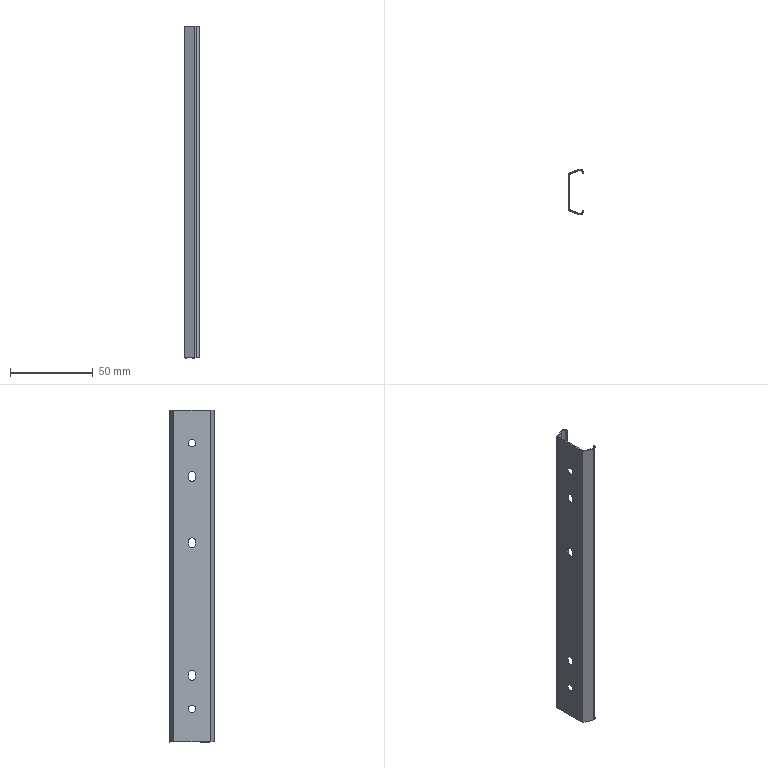Part | SolidWorks | features BaseBody 1 | 1 solid | 37 faces | box 9 x 27 x 200 mm | volume 4310 mm3 | plane 20 | cylinder 17 | commonest cylinder face diameters 4.2 x9 3.7 x4 4.5 x4
STEP:
#1=CARTESIAN_POINT('',(-2.5,11.15,17.75));
#2=VERTEX_POINT('',#1);
#3=CARTESIAN_POINT('',(-2.5,11.15,22.25));
#4=VERTEX_POINT('',#3);
#5=CARTESIAN_POINT('',(-2.5,11.15,20.));
#6=DIRECTION('',(-1.,0.,0.));
#7=DIRECTION('',(0.,0.,1.));
#8=AXIS2_PLACEMENT_3D('',#5,#6,#7);
#9=CIRCLE('',#8,2.25);
#10=EDGE_CURVE('',#2,#4,#9,.T.);
#11=ORIENTED_EDGE('',*,*,#10,.F.);
#12=CARTESIAN_POINT('',(-3.,11.15,17.75));
#13=VERTEX_POINT('',#12);
#14=CARTESIAN_POINT('',(-3.,11.15,17.75));
#15=DIRECTION('',(-1.,0.,0.));
#16=VECTOR('',#15,1000.);
#17=LINE('',#14,#16);
#18=EDGE_CURVE('',#2,#13,#17,.T.);
#19=ORIENTED_EDGE('',*,*,#18,.T.);
#20=CARTESIAN_POINT('',(-3.,11.15,22.25));
#21=VERTEX_POINT('',#20);
#22=CARTESIAN_POINT('',(-3.,11.15,20.));
#23=DIRECTION('',(1.,0.,0.));
#24=DIRECTION('',(0.,0.,1.));
#25=AXIS2_PLACEMENT_3D('',#22,#23,#24);
#26=CIRCLE('',#25,2.25);
#27=EDGE_CURVE('',#21,#13,#26,.T.);
#28=ORIENTED_EDGE('',*,*,#27,.F.);
#29=CARTESIAN_POINT('',(-3.,11.15,22.25));
#30=DIRECTION('',(-1.,0.,0.));
#31=VECTOR('',#30,1000.);
#32=LINE('',#29,#31);
#33=EDGE_CURVE('',#4,#21,#32,.T.);
#34=ORIENTED_EDGE('',*,*,#33,.F.);
#35=EDGE_LOOP('',(#11,#19,#28,#34));
#36=FACE_OUTER_BOUND('',#35,.T.);
#37=CARTESIAN_POINT('',(-3.,11.15,20.));
#38=DIRECTION('',(-1.,0.,0.));
#39=DIRECTION('',(0.,0.,1.));
#40=AXIS2_PLACEMENT_3D('',#37,#38,#39);
#41=CYLINDRICAL_SURFACE('',#40,2.25);
#42=ADVANCED_FACE('',(#36),#41,.F.);
#43=CARTESIAN_POINT('',(-2.5,11.15,177.75));
#44=VERTEX_POINT('',#43);
#45=CARTESIAN_POINT('',(-2.5,11.15,182.25));
#46=VERTEX_POINT('',#45);
#47=CARTESIAN_POINT('',(-2.5,11.15,180.));
#48=DIRECTION('',(-1.,0.,0.));
#49=DIRECTION('',(0.,0.,1.));
#50=AXIS2_PLACEMENT_3D('',#47,#48,#49);
#51=CIRCLE('',#50,2.25);
#52=EDGE_CURVE('',#44,#46,#51,.T.);
#53=ORIENTED_EDGE('',*,*,#52,.F.);
#54=CARTESIAN_POINT('',(-3.,11.15,177.75));
#55=VERTEX_POINT('',#54);
#56=CARTESIAN_POINT('',(-3.,11.15,177.75));
#57=DIRECTION('',(-1.,0.,0.));
#58=VECTOR('',#57,1000.);
#59=LINE('',#56,#58);
#60=EDGE_CURVE('',#44,#55,#59,.T.);
#61=ORIENTED_EDGE('',*,*,#60,.T.);
#62=CARTESIAN_POINT('',(-3.,11.15,182.25));
#63=VERTEX_POINT('',#62);
#64=CARTESIAN_POINT('',(-3.,11.15,180.));
#65=DIRECTION('',(1.,0.,0.));
#66=DIRECTION('',(0.,0.,1.));
#67=AXIS2_PLACEMENT_3D('',#64,#65,#66);
#68=CIRCLE('',#67,2.25);
#69=EDGE_CURVE('',#63,#55,#68,.T.);
#70=ORIENTED_EDGE('',*,*,#69,.F.);
#71=CARTESIAN_POINT('',(-3.,11.15,182.25));
#72=DIRECTION('',(-1.,0.,0.));
#73=VECTOR('',#72,1000.);
#74=LINE('',#71,#73);
#75=EDGE_CURVE('',#46,#63,#74,.T.);
#76=ORIENTED_EDGE('',*,*,#75,.F.);
#77=EDGE_LOOP('',(#53,#61,#70,#76));
#78=FACE_OUTER_BOUND('',#77,.T.);
#79=CARTESIAN_POINT('',(-3.,11.15,180.));
#80=DIRECTION('',(-1.,0.,0.));
#81=DIRECTION('',(0.,0.,1.));
#82=AXIS2_PLACEMENT_3D('',#79,#80,#81);
#83=CYLINDRICAL_SURFACE('',#82,2.25);
#84=ADVANCED_FACE('',(#78),#83,.F.);
#85=CARTESIAN_POINT('',(-2.5,11.15,43.));
#86=VERTEX_POINT('',#85);
#87=CARTESIAN_POINT('',(-2.5,13.25,40.9));
#88=VERTEX_POINT('',#87);
#89=CARTESIAN_POINT('',(-2.5,11.15,40.9));
#90=DIRECTION('',(-1.,0.,0.));
#91=DIRECTION('',(0.,0.,1.));
#92=AXIS2_PLACEMENT_3D('',#89,#90,#91);
#93=CIRCLE('',#92,2.1);
#94=EDGE_CURVE('',#86,#88,#93,.T.);
#95=ORIENTED_EDGE('',*,*,#94,.F.);
#96=CARTESIAN_POINT('',(-3.,11.15,43.));
#97=VERTEX_POINT('',#96);
#98=CARTESIAN_POINT('',(-3.,11.15,43.));
#99=DIRECTION('',(-1.,0.,0.));
#100=VECTOR('',#99,1000.);
#101=LINE('',#98,#100);
#102=EDGE_CURVE('',#86,#97,#101,.T.);
#103=ORIENTED_EDGE('',*,*,#102,.T.);
#104=CARTESIAN_POINT('',(-3.,13.25,40.9));
#105=VERTEX_POINT('',#104);
#106=CARTESIAN_POINT('',(-3.,11.15,40.9));
#107=DIRECTION('',(1.,0.,0.));
#108=DIRECTION('',(0.,0.,1.));
#109=AXIS2_PLACEMENT_3D('',#106,#107,#108);
#110=CIRCLE('',#109,2.1);
#111=EDGE_CURVE('',#105,#97,#110,.T.);
#112=ORIENTED_EDGE('',*,*,#111,.F.);
#113=CARTESIAN_POINT('',(-3.,13.25,40.9));
#114=DIRECTION('',(-1.,0.,0.));
#115=VECTOR('',#114,1000.);
#116=LINE('',#113,#115);
#117=EDGE_CURVE('',#88,#105,#116,.T.);
#118=ORIENTED_EDGE('',*,*,#117,.F.);
#119=EDGE_LOOP('',(#95,#103,#112,#118));
#120=FACE_OUTER_BOUND('',#119,.T.);
#121=CARTESIAN_POINT('',(-3.,11.15,40.9));
#122=DIRECTION('',(-1.,0.,0.));
#123=DIRECTION('',(0.,0.,1.));
#124=AXIS2_PLACEMENT_3D('',#121,#122,#123);
#125=CYLINDRICAL_SURFACE('',#124,2.1);
#126=ADVANCED_FACE('',(#120),#125,.F.);
#127=CARTESIAN_POINT('',(-2.5,11.15,163.));
#128=VERTEX_POINT('',#127);
#129=CARTESIAN_POINT('',(-2.5,13.25,160.9));
#130=VERTEX_POINT('',#129);
#131=CARTESIAN_POINT('',(-2.5,11.15,160.9));
#132=DIRECTION('',(-1.,0.,0.));
#133=DIRECTION('',(0.,0.,1.));
#134=AXIS2_PLACEMENT_3D('',#131,#132,#133);
#135=CIRCLE('',#134,2.1);
#136=EDGE_CURVE('',#128,#130,#135,.T.);
#137=ORIENTED_EDGE('',*,*,#136,.F.);
#138=CARTESIAN_POINT('',(-3.,11.15,163.));
#139=VERTEX_POINT('',#138);
#140=CARTESIAN_POINT('',(-3.,11.15,163.));
#141=DIRECTION('',(-1.,0.,0.));
#142=VECTOR('',#141,1000.);
#143=LINE('',#140,#142);
#144=EDGE_CURVE('',#128,#139,#143,.T.);
#145=ORIENTED_EDGE('',*,*,#144,.T.);
#146=CARTESIAN_POINT('',(-3.,13.25,160.9));
#147=VERTEX_POINT('',#146);
#148=CARTESIAN_POINT('',(-3.,11.15,160.9));
#149=DIRECTION('',(1.,0.,0.));
#150=DIRECTION('',(0.,0.,1.));
#151=AXIS2_PLACEMENT_3D('',#148,#149,#150);
#152=CIRCLE('',#151,2.1);
#153=EDGE_CURVE('',#147,#139,#152,.T.);
#154=ORIENTED_EDGE('',*,*,#153,.F.);
#155=CARTESIAN_POINT('',(-3.,13.25,160.9));
#156=DIRECTION('',(-1.,0.,0.));
#157=VECTOR('',#156,1000.);
#158=LINE('',#155,#157);
#159=EDGE_CURVE('',#130,#147,#158,.T.);
#160=ORIENTED_EDGE('',*,*,#159,.F.);
#161=EDGE_LOOP('',(#137,#145,#154,#160));
#162=FACE_OUTER_BOUND('',#161,.T.);
#163=CARTESIAN_POINT('',(-3.,11.15,160.9));
#164=DIRECTION('',(-1.,0.,0.));
#165=DIRECTION('',(0.,0.,1.));
#166=AXIS2_PLACEMENT_3D('',#163,#164,#165);
#167=CYLINDRICAL_SURFACE('',#166,2.1);
#168=ADVANCED_FACE('',(#162),#167,.F.);
#169=CARTESIAN_POINT('',(-2.5,11.15,123.));
#170=VERTEX_POINT('',#169);
#171=CARTESIAN_POINT('',(-2.5,13.25,120.9));
#172=VERTEX_POINT('',#171);
#173=CARTESIAN_POINT('',(-2.5,11.15,120.9));
#174=DIRECTION('',(-1.,0.,0.));
#175=DIRECTION('',(0.,0.,1.));
#176=AXIS2_PLACEMENT_3D('',#173,#174,#175);
#177=CIRCLE('',#176,2.1);
#178=EDGE_CURVE('',#170,#172,#177,.T.);
#179=ORIENTED_EDGE('',*,*,#178,.F.);
#180=CARTESIAN_POINT('',(-3.,11.15,123.));
#181=VERTEX_POINT('',#180);
#182=CARTESIAN_POINT('',(-3.,11.15,123.));
#183=DIRECTION('',(-1.,0.,0.));
#184=VECTOR('',#183,1000.);
#185=LINE('',#182,#184);
#186=EDGE_CURVE('',#170,#181,#185,.T.);
#187=ORIENTED_EDGE('',*,*,#186,.T.);
#188=CARTESIAN_POINT('',(-3.,13.25,120.9));
#189=VERTEX_POINT('',#188);
#190=CARTESIAN_POINT('',(-3.,11.15,120.9));
#191=DIRECTION('',(1.,0.,0.));
#192=DIRECTION('',(0.,0.,1.));
#193=AXIS2_PLACEMENT_3D('',#190,#191,#192);
#194=CIRCLE('',#193,2.1);
#195=EDGE_CURVE('',#189,#181,#194,.T.);
#196=ORIENTED_EDGE('',*,*,#195,.F.);
#197=CARTESIAN_POINT('',(-3.,13.25,120.9));
#198=DIRECTION('',(-1.,0.,0.));
#199=VECTOR('',#198,1000.);
#200=LINE('',#197,#199);
#201=EDGE_CURVE('',#172,#189,#200,.T.);
#202=ORIENTED_EDGE('',*,*,#201,.F.);
#203=EDGE_LOOP('',(#179,#187,#196,#202));
#204=FACE_OUTER_BOUND('',#203,.T.);
#205=CARTESIAN_POINT('',(-3.,11.15,120.9));
#206=DIRECTION('',(-1.,0.,0.));
#207=DIRECTION('',(0.,0.,1.));
#208=AXIS2_PLACEMENT_3D('',#205,#206,#207);
#209=CYLINDRICAL_SURFACE('',#208,2.1);
#210=ADVANCED_FACE('',(#204),#209,.F.);
#211=CARTESIAN_POINT('',(-3.,0.05325,200.));
#212=VERTEX_POINT('',#211);
#213=CARTESIAN_POINT('',(-3.,22.247,200.));
#214=VERTEX_POINT('',#213);
#215=CARTESIAN_POINT('',(-3.,22.247,200.));
#216=DIRECTION('',(0.,1.,0.));
#217=VECTOR('',#216,1000.);
#218=LINE('',#215,#217);
#219=EDGE_CURVE('',#212,#214,#218,.T.);
#220=ORIENTED_EDGE('',*,*,#219,.T.);
#221=CARTESIAN_POINT('',(-3.,22.247,0.));
#222=VERTEX_POINT('',#221);
#223=CARTESIAN_POINT('',(-3.,22.247,200.));
#224=DIRECTION('',(0.,0.,-1.));
#225=VECTOR('',#224,1000.);
#226=LINE('',#223,#225);
#227=EDGE_CURVE('',#214,#222,#226,.T.);
#228=ORIENTED_EDGE('',*,*,#227,.T.);
#229=CARTESIAN_POINT('',(-3.,0.05325,0.));
#230=VERTEX_POINT('',#229);
#231=CARTESIAN_POINT('',(-3.,22.247,0.));
#232=DIRECTION('',(0.,-1.,0.));
#233=VECTOR('',#232,1000.);
#234=LINE('',#231,#233);
#235=EDGE_CURVE('',#222,#230,#234,.T.);
#236=ORIENTED_EDGE('',*,*,#235,.T.);
#237=CARTESIAN_POINT('',(-3.,0.05325,200.));
#238=DIRECTION('',(0.,0.,1.));
#239=VECTOR('',#238,1000.);
#240=LINE('',#237,#239);
#241=EDGE_CURVE('',#230,#212,#240,.T.);
#242=ORIENTED_EDGE('',*,*,#241,.T.);
#243=EDGE_LOOP('',(#220,#228,#236,#242));
#244=FACE_OUTER_BOUND('',#243,.T.);
#245=ORIENTED_EDGE('',*,*,#27,.T.);
#246=CARTESIAN_POINT('',(-3.,11.15,20.));
#247=DIRECTION('',(1.,0.,0.));
#248=DIRECTION('',(0.,0.,1.));
#249=AXIS2_PLACEMENT_3D('',#246,#247,#248);
#250=CIRCLE('',#249,2.25);
#251=EDGE_CURVE('',#13,#21,#250,.T.);
#252=ORIENTED_EDGE('',*,*,#251,.T.);
#253=EDGE_LOOP('',(#245,#252));
#254=FACE_BOUND('',#253,.T.);
#255=ORIENTED_EDGE('',*,*,#69,.T.);
#256=CARTESIAN_POINT('',(-3.,11.15,180.));
#257=DIRECTION('',(1.,0.,0.));
#258=DIRECTION('',(0.,0.,1.));
#259=AXIS2_PLACEMENT_3D('',#256,#257,#258);
#260=CIRCLE('',#259,2.25);
#261=EDGE_CURVE('',#55,#63,#260,.T.);
#262=ORIENTED_EDGE('',*,*,#261,.T.);
#263=EDGE_LOOP('',(#255,#262));
#264=FACE_BOUND('',#263,.T.);
#265=ORIENTED_EDGE('',*,*,#111,.T.);
#266=CARTESIAN_POINT('',(-3.,9.05,40.9));
#267=VERTEX_POINT('',#266);
#268=CARTESIAN_POINT('',(-3.,11.15,40.9));
#269=DIRECTION('',(1.,0.,0.));
#270=DIRECTION('',(0.,0.,1.));
#271=AXIS2_PLACEMENT_3D('',#268,#269,#270);
#272=CIRCLE('',#271,2.1);
#273=EDGE_CURVE('',#97,#267,#272,.T.);
#274=ORIENTED_EDGE('',*,*,#273,.T.);
#275=CARTESIAN_POINT('',(-3.,9.05,39.1));
#276=VERTEX_POINT('',#275);
#277=CARTESIAN_POINT('',(-3.,9.05,200.));
#278=DIRECTION('',(0.,0.,-1.));
#279=VECTOR('',#278,1000.);
#280=LINE('',#277,#279);
#281=EDGE_CURVE('',#267,#276,#280,.T.);
#282=ORIENTED_EDGE('',*,*,#281,.T.);
#283=CARTESIAN_POINT('',(-3.,13.25,39.1));
#284=VERTEX_POINT('',#283);
#285=CARTESIAN_POINT('',(-3.,11.15,39.1));
#286=DIRECTION('',(1.,0.,0.));
#287=DIRECTION('',(0.,0.,1.));
#288=AXIS2_PLACEMENT_3D('',#285,#286,#287);
#289=CIRCLE('',#288,2.1);
#290=EDGE_CURVE('',#276,#284,#289,.T.);
#291=ORIENTED_EDGE('',*,*,#290,.T.);
#292=CARTESIAN_POINT('',(-3.,13.25,200.));
#293=DIRECTION('',(0.,0.,1.));
#294=VECTOR('',#293,1000.);
#295=LINE('',#292,#294);
#296=EDGE_CURVE('',#284,#105,#295,.T.);
#297=ORIENTED_EDGE('',*,*,#296,.T.);
#298=EDGE_LOOP('',(#265,#274,#282,#291,#297));
#299=FACE_BOUND('',#298,.T.);
#300=ORIENTED_EDGE('',*,*,#153,.T.);
#301=CARTESIAN_POINT('',(-3.,9.05,160.9));
#302=VERTEX_POINT('',#301);
#303=CARTESIAN_POINT('',(-3.,11.15,160.9));
#304=DIRECTION('',(1.,0.,0.));
#305=DIRECTION('',(0.,0.,1.));
#306=AXIS2_PLACEMENT_3D('',#303,#304,#305);
#307=CIRCLE('',#306,2.1);
#308=EDGE_CURVE('',#139,#302,#307,.T.);
#309=ORIENTED_EDGE('',*,*,#308,.T.);
#310=CARTESIAN_POINT('',(-3.,9.05,159.1));
#311=VERTEX_POINT('',#310);
#312=CARTESIAN_POINT('',(-3.,9.05,200.));
#313=DIRECTION('',(0.,0.,-1.));
#314=VECTOR('',#313,1000.);
#315=LINE('',#312,#314);
#316=EDGE_CURVE('',#302,#311,#315,.T.);
#317=ORIENTED_EDGE('',*,*,#316,.T.);
#318=CARTESIAN_POINT('',(-3.,13.25,159.1));
#319=VERTEX_POINT('',#318);
#320=CARTESIAN_POINT('',(-3.,11.15,159.1));
#321=DIRECTION('',(1.,0.,0.));
#322=DIRECTION('',(0.,0.,1.));
#323=AXIS2_PLACEMENT_3D('',#320,#321,#322);
#324=CIRCLE('',#323,2.1);
#325=EDGE_CURVE('',#311,#319,#324,.T.);
#326=ORIENTED_EDGE('',*,*,#325,.T.);
#327=CARTESIAN_POINT('',(-3.,13.25,200.));
#328=DIRECTION('',(0.,0.,1.));
#329=VECTOR('',#328,1000.);
#330=LINE('',#327,#329);
#331=EDGE_CURVE('',#319,#147,#330,.T.);
#332=ORIENTED_EDGE('',*,*,#331,.T.);
#333=EDGE_LOOP('',(#300,#309,#317,#326,#332));
#334=FACE_BOUND('',#333,.T.);
#335=ORIENTED_EDGE('',*,*,#195,.T.);
#336=CARTESIAN_POINT('',(-3.,9.05,120.9));
#337=VERTEX_POINT('',#336);
#338=CARTESIAN_POINT('',(-3.,11.15,120.9));
#339=DIRECTION('',(1.,0.,0.));
#340=DIRECTION('',(0.,0.,1.));
#341=AXIS2_PLACEMENT_3D('',#338,#339,#340);
#342=CIRCLE('',#341,2.1);
#343=EDGE_CURVE('',#181,#337,#342,.T.);
#344=ORIENTED_EDGE('',*,*,#343,.T.);
#345=CARTESIAN_POINT('',(-3.,9.05,119.1));
#346=VERTEX_POINT('',#345);
#347=CARTESIAN_POINT('',(-3.,9.05,200.));
#348=DIRECTION('',(0.,0.,-1.));
#349=VECTOR('',#348,1000.);
#350=LINE('',#347,#349);
#351=EDGE_CURVE('',#337,#346,#350,.T.);
#352=ORIENTED_EDGE('',*,*,#351,.T.);
#353=CARTESIAN_POINT('',(-3.,13.25,119.1));
#354=VERTEX_POINT('',#353);
#355=CARTESIAN_POINT('',(-3.,11.15,119.1));
#356=DIRECTION('',(1.,0.,0.));
#357=DIRECTION('',(0.,0.,1.));
#358=AXIS2_PLACEMENT_3D('',#355,#356,#357);
#359=CIRCLE('',#358,2.1);
#360=EDGE_CURVE('',#346,#354,#359,.T.);
#361=ORIENTED_EDGE('',*,*,#360,.T.);
#362=CARTESIAN_POINT('',(-3.,13.25,200.));
#363=DIRECTION('',(0.,0.,1.));
#364=VECTOR('',#363,1000.);
#365=LINE('',#362,#364);
#366=EDGE_CURVE('',#354,#189,#365,.T.);
#367=ORIENTED_EDGE('',*,*,#366,.T.);
#368=EDGE_LOOP('',(#335,#344,#352,#361,#367));
#369=FACE_BOUND('',#368,.T.);
#370=CARTESIAN_POINT('',(-3.,22.247,200.));
#371=DIRECTION('',(-1.,0.,0.));
#372=DIRECTION('',(0.,0.,1.));
#373=AXIS2_PLACEMENT_3D('',#370,#371,#372);
#374=PLANE('',#373);
#375=ADVANCED_FACE('',(#244,#254,#264,#299,#334,#369),#374,.T.);
#376=CARTESIAN_POINT('',(3.211,24.65,200.));
#377=VERTEX_POINT('',#376);
#378=CARTESIAN_POINT('',(3.211,24.65,200.));
#379=DIRECTION('',(0.9326,0.3609,0.));
#380=VECTOR('',#379,1000.);
#381=LINE('',#378,#380);
#382=EDGE_CURVE('',#214,#377,#381,.T.);
#383=ORIENTED_EDGE('',*,*,#382,.T.);
#384=CARTESIAN_POINT('',(3.211,24.65,0.));
#385=VERTEX_POINT('',#384);
#386=CARTESIAN_POINT('',(3.211,24.65,200.));
#387=DIRECTION('',(0.,0.,-1.));
#388=VECTOR('',#387,1000.);
#389=LINE('',#386,#388);
#390=EDGE_CURVE('',#377,#385,#389,.T.);
#391=ORIENTED_EDGE('',*,*,#390,.T.);
#392=CARTESIAN_POINT('',(3.211,24.65,0.));
#393=DIRECTION('',(-0.9326,-0.3609,0.));
#394=VECTOR('',#393,1000.);
#395=LINE('',#392,#394);
#396=EDGE_CURVE('',#385,#222,#395,.T.);
#397=ORIENTED_EDGE('',*,*,#396,.T.);
#398=ORIENTED_EDGE('',*,*,#227,.F.);
#399=EDGE_LOOP('',(#383,#391,#397,#398));
#400=FACE_OUTER_BOUND('',#399,.T.);
#401=CARTESIAN_POINT('',(3.211,24.65,200.));
#402=DIRECTION('',(-0.3609,0.9326,0.));
#403=DIRECTION('',(-0.9326,-0.3609,0.));
#404=AXIS2_PLACEMENT_3D('',#401,#402,#403);
#405=PLANE('',#404);
#406=ADVANCED_FACE('',(#400),#405,.T.);
#407=CARTESIAN_POINT('',(3.211,-2.35,200.));
#408=VERTEX_POINT('',#407);
#409=CARTESIAN_POINT('',(3.211,-2.35,200.));
#410=DIRECTION('',(-0.9326,0.3609,0.));
#411=VECTOR('',#410,1000.);
#412=LINE('',#409,#411);
#413=EDGE_CURVE('',#408,#212,#412,.T.);
#414=ORIENTED_EDGE('',*,*,#413,.F.);
#415=CARTESIAN_POINT('',(4.15,-2.35,200.));
#416=VERTEX_POINT('',#415);
#417=CARTESIAN_POINT('',(3.211,-2.35,200.));
#418=DIRECTION('',(-1.,0.,0.));
#419=VECTOR('',#418,1000.);
#420=LINE('',#417,#419);
#421=EDGE_CURVE('',#416,#408,#420,.T.);
#422=ORIENTED_EDGE('',*,*,#421,.F.);
#423=CARTESIAN_POINT('',(6.,-0.5,200.));
#424=VERTEX_POINT('',#423);
#425=CARTESIAN_POINT('',(4.15,-0.5,200.));
#426=DIRECTION('',(0.,0.,-1.));
#427=DIRECTION('',(1.,0.,0.));
#428=AXIS2_PLACEMENT_3D('',#425,#426,#427);
#429=CIRCLE('',#428,1.85);
#430=EDGE_CURVE('',#424,#416,#429,.T.);
#431=ORIENTED_EDGE('',*,*,#430,.F.);
#432=CARTESIAN_POINT('',(6.,-0.2056,200.));
#433=VERTEX_POINT('',#432);
#434=CARTESIAN_POINT('',(6.,-0.5,200.));
#435=DIRECTION('',(0.,-1.,0.));
#436=VECTOR('',#435,1000.);
#437=LINE('',#434,#436);
#438=EDGE_CURVE('',#433,#424,#437,.T.);
#439=ORIENTED_EDGE('',*,*,#438,.F.);
#440=CARTESIAN_POINT('',(5.493,-0.1612,200.));
#441=VERTEX_POINT('',#440);
#442=CARTESIAN_POINT('',(6.,-0.2056,200.));
#443=DIRECTION('',(0.9962,-0.08716,0.));
#444=VECTOR('',#443,1000.);
#445=LINE('',#442,#444);
#446=EDGE_CURVE('',#441,#433,#445,.T.);
#447=ORIENTED_EDGE('',*,*,#446,.F.);
#448=CARTESIAN_POINT('',(2.982,-1.725,200.));
#449=VERTEX_POINT('',#448);
#450=CARTESIAN_POINT('',(3.65,0.,200.));
#451=DIRECTION('',(0.,0.,1.));
#452=DIRECTION('',(1.,0.,0.));
#453=AXIS2_PLACEMENT_3D('',#450,#451,#452);
#454=CIRCLE('',#453,1.85);
#455=EDGE_CURVE('',#449,#441,#454,.T.);
#456=ORIENTED_EDGE('',*,*,#455,.F.);
#457=CARTESIAN_POINT('',(-2.5,0.3959,200.));
#458=VERTEX_POINT('',#457);
#459=CARTESIAN_POINT('',(-2.5,0.3959,200.));
#460=DIRECTION('',(0.9326,-0.3609,0.));
#461=VECTOR('',#460,1000.);
#462=LINE('',#459,#461);
#463=EDGE_CURVE('',#458,#449,#462,.T.);
#464=ORIENTED_EDGE('',*,*,#463,.F.);
#465=CARTESIAN_POINT('',(-2.5,21.904,200.));
#466=VERTEX_POINT('',#465);
#467=CARTESIAN_POINT('',(-2.5,24.65,200.));
#468=DIRECTION('',(0.,-1.,0.));
#469=VECTOR('',#468,1000.);
#470=LINE('',#467,#469);
#471=EDGE_CURVE('',#466,#458,#470,.T.);
#472=ORIENTED_EDGE('',*,*,#471,.F.);
#473=CARTESIAN_POINT('',(2.982,24.025,200.));
#474=VERTEX_POINT('',#473);
#475=CARTESIAN_POINT('',(2.982,24.025,200.));
#476=DIRECTION('',(-0.9326,-0.3609,0.));
#477=VECTOR('',#476,1000.);
#478=LINE('',#475,#477);
#479=EDGE_CURVE('',#474,#466,#478,.T.);
#480=ORIENTED_EDGE('',*,*,#479,.F.);
#481=CARTESIAN_POINT('',(5.493,22.461,200.));
#482=VERTEX_POINT('',#481);
#483=CARTESIAN_POINT('',(3.65,22.3,200.));
#484=DIRECTION('',(0.,0.,1.));
#485=DIRECTION('',(1.,0.,0.));
#486=AXIS2_PLACEMENT_3D('',#483,#484,#485);
#487=CIRCLE('',#486,1.85);
#488=EDGE_CURVE('',#482,#474,#487,.T.);
#489=ORIENTED_EDGE('',*,*,#488,.F.);
#490=CARTESIAN_POINT('',(6.,22.506,200.));
#491=VERTEX_POINT('',#490);
#492=CARTESIAN_POINT('',(5.493,22.461,200.));
#493=DIRECTION('',(-0.9962,-0.08716,0.));
#494=VECTOR('',#493,1000.);
#495=LINE('',#492,#494);
#496=EDGE_CURVE('',#491,#482,#495,.T.);
#497=ORIENTED_EDGE('',*,*,#496,.F.);
#498=CARTESIAN_POINT('',(6.,22.8,200.));
#499=VERTEX_POINT('',#498);
#500=CARTESIAN_POINT('',(6.,22.506,200.));
#501=DIRECTION('',(0.,-1.,0.));
#502=VECTOR('',#501,1000.);
#503=LINE('',#500,#502);
#504=EDGE_CURVE('',#499,#491,#503,.T.);
#505=ORIENTED_EDGE('',*,*,#504,.F.);
#506=CARTESIAN_POINT('',(4.15,24.65,200.));
#507=VERTEX_POINT('',#506);
#508=CARTESIAN_POINT('',(4.15,22.8,200.));
#509=DIRECTION('',(0.,0.,-1.));
#510=DIRECTION('',(1.,0.,0.));
#511=AXIS2_PLACEMENT_3D('',#508,#509,#510);
#512=CIRCLE('',#511,1.85);
#513=EDGE_CURVE('',#507,#499,#512,.T.);
#514=ORIENTED_EDGE('',*,*,#513,.F.);
#515=CARTESIAN_POINT('',(-3.,24.65,200.));
#516=DIRECTION('',(1.,0.,0.));
#517=VECTOR('',#516,1000.);
#518=LINE('',#515,#517);
#519=EDGE_CURVE('',#377,#507,#518,.T.);
#520=ORIENTED_EDGE('',*,*,#519,.F.);
#521=ORIENTED_EDGE('',*,*,#382,.F.);
#522=ORIENTED_EDGE('',*,*,#219,.F.);
#523=EDGE_LOOP('',(#414,#422,#431,#439,#447,#456,#464,#472,#480,#489,#497,#505,#514,#520,#521,#522));
#524=FACE_OUTER_BOUND('',#523,.T.);
#525=CARTESIAN_POINT('',(-3.,24.65,200.));
#526=DIRECTION('',(0.,0.,-1.));
#527=DIRECTION('',(-1.,0.,0.));
#528=AXIS2_PLACEMENT_3D('',#525,#526,#527);
#529=PLANE('',#528);
#530=ADVANCED_FACE('',(#524),#529,.F.);
#531=ORIENTED_EDGE('',*,*,#413,.T.);
#532=ORIENTED_EDGE('',*,*,#241,.F.);
#533=CARTESIAN_POINT('',(3.211,-2.35,0.));
#534=VERTEX_POINT('',#533);
#535=CARTESIAN_POINT('',(-3.,0.05325,0.));
#536=DIRECTION('',(0.9326,-0.3609,0.));
#537=VECTOR('',#536,1000.);
#538=LINE('',#535,#537);
#539=EDGE_CURVE('',#230,#534,#538,.T.);
#540=ORIENTED_EDGE('',*,*,#539,.T.);
#541=CARTESIAN_POINT('',(3.211,-2.35,200.));
#542=DIRECTION('',(0.,0.,1.));
#543=VECTOR('',#542,1000.);
#544=LINE('',#541,#543);
#545=EDGE_CURVE('',#534,#408,#544,.T.);
#546=ORIENTED_EDGE('',*,*,#545,.T.);
#547=EDGE_LOOP('',(#531,#532,#540,#546));
#548=FACE_OUTER_BOUND('',#547,.T.);
#549=CARTESIAN_POINT('',(-3.,0.05325,200.));
#550=DIRECTION('',(-0.3609,-0.9326,0.));
#551=DIRECTION('',(0.9326,-0.3609,0.));
#552=AXIS2_PLACEMENT_3D('',#549,#550,#551);
#553=PLANE('',#552);
#554=ADVANCED_FACE('',(#548),#553,.T.);
#555=CARTESIAN_POINT('',(6.,-0.5,0.));
#556=VERTEX_POINT('',#555);
#557=CARTESIAN_POINT('',(4.15,-2.35,0.));
#558=VERTEX_POINT('',#557);
#559=CARTESIAN_POINT('',(4.15,-0.5,0.));
#560=DIRECTION('',(0.,0.,-1.));
#561=DIRECTION('',(1.,0.,0.));
#562=AXIS2_PLACEMENT_3D('',#559,#560,#561);
#563=CIRCLE('',#562,1.85);
#564=EDGE_CURVE('',#556,#558,#563,.T.);
#565=ORIENTED_EDGE('',*,*,#564,.T.);
#566=CARTESIAN_POINT('',(-3.,-2.35,0.));
#567=DIRECTION('',(-1.,0.,0.));
#568=VECTOR('',#567,1000.);
#569=LINE('',#566,#568);
#570=EDGE_CURVE('',#558,#534,#569,.T.);
#571=ORIENTED_EDGE('',*,*,#570,.T.);
#572=ORIENTED_EDGE('',*,*,#539,.F.);
#573=ORIENTED_EDGE('',*,*,#235,.F.);
#574=ORIENTED_EDGE('',*,*,#396,.F.);
#575=CARTESIAN_POINT('',(4.15,24.65,0.));
#576=VERTEX_POINT('',#575);
#577=CARTESIAN_POINT('',(-3.,24.65,0.));
#578=DIRECTION('',(1.,0.,0.));
#579=VECTOR('',#578,1000.);
#580=LINE('',#577,#579);
#581=EDGE_CURVE('',#385,#576,#580,.T.);
#582=ORIENTED_EDGE('',*,*,#581,.T.);
#583=CARTESIAN_POINT('',(6.,22.8,0.));
#584=VERTEX_POINT('',#583);
#585=CARTESIAN_POINT('',(4.15,22.8,0.));
#586=DIRECTION('',(0.,0.,-1.));
#587=DIRECTION('',(1.,0.,0.));
#588=AXIS2_PLACEMENT_3D('',#585,#586,#587);
#589=CIRCLE('',#588,1.85);
#590=EDGE_CURVE('',#576,#584,#589,.T.);
#591=ORIENTED_EDGE('',*,*,#590,.T.);
#592=CARTESIAN_POINT('',(6.,22.506,0.));
#593=VERTEX_POINT('',#592);
#594=CARTESIAN_POINT('',(6.,22.506,0.));
#595=DIRECTION('',(0.,1.,0.));
#596=VECTOR('',#595,1000.);
#597=LINE('',#594,#596);
#598=EDGE_CURVE('',#593,#584,#597,.T.);
#599=ORIENTED_EDGE('',*,*,#598,.F.);
#600=CARTESIAN_POINT('',(5.493,22.461,0.));
#601=VERTEX_POINT('',#600);
#602=CARTESIAN_POINT('',(5.493,22.461,0.));
#603=DIRECTION('',(0.9962,0.08716,0.));
#604=VECTOR('',#603,1000.);
#605=LINE('',#602,#604);
#606=EDGE_CURVE('',#601,#593,#605,.T.);
#607=ORIENTED_EDGE('',*,*,#606,.F.);
#608=CARTESIAN_POINT('',(2.982,24.025,0.));
#609=VERTEX_POINT('',#608);
#610=CARTESIAN_POINT('',(3.65,22.3,0.));
#611=DIRECTION('',(0.,0.,1.));
#612=DIRECTION('',(1.,0.,0.));
#613=AXIS2_PLACEMENT_3D('',#610,#611,#612);
#614=CIRCLE('',#613,1.85);
#615=EDGE_CURVE('',#601,#609,#614,.T.);
#616=ORIENTED_EDGE('',*,*,#615,.T.);
#617=CARTESIAN_POINT('',(-2.5,21.904,0.));
#618=VERTEX_POINT('',#617);
#619=CARTESIAN_POINT('',(2.982,24.025,0.));
#620=DIRECTION('',(-0.9326,-0.3609,0.));
#621=VECTOR('',#620,1000.);
#622=LINE('',#619,#621);
#623=EDGE_CURVE('',#609,#618,#622,.T.);
#624=ORIENTED_EDGE('',*,*,#623,.T.);
#625=CARTESIAN_POINT('',(-2.5,0.3959,0.));
#626=VERTEX_POINT('',#625);
#627=CARTESIAN_POINT('',(-2.5,24.65,0.));
#628=DIRECTION('',(0.,-1.,0.));
#629=VECTOR('',#628,1000.);
#630=LINE('',#627,#629);
#631=EDGE_CURVE('',#618,#626,#630,.T.);
#632=ORIENTED_EDGE('',*,*,#631,.T.);
#633=CARTESIAN_POINT('',(2.982,-1.725,0.));
#634=VERTEX_POINT('',#633);
#635=CARTESIAN_POINT('',(-2.5,0.3959,0.));
#636=DIRECTION('',(0.9326,-0.3609,0.));
#637=VECTOR('',#636,1000.);
#638=LINE('',#635,#637);
#639=EDGE_CURVE('',#626,#634,#638,.T.);
#640=ORIENTED_EDGE('',*,*,#639,.T.);
#641=CARTESIAN_POINT('',(5.493,-0.1612,0.));
#642=VERTEX_POINT('',#641);
#643=CARTESIAN_POINT('',(3.65,0.,0.));
#644=DIRECTION('',(0.,0.,1.));
#645=DIRECTION('',(1.,0.,0.));
#646=AXIS2_PLACEMENT_3D('',#643,#644,#645);
#647=CIRCLE('',#646,1.85);
#648=EDGE_CURVE('',#634,#642,#647,.T.);
#649=ORIENTED_EDGE('',*,*,#648,.T.);
#650=CARTESIAN_POINT('',(6.,-0.2056,0.));
#651=VERTEX_POINT('',#650);
#652=CARTESIAN_POINT('',(6.,-0.2056,0.));
#653=DIRECTION('',(-0.9962,0.08716,0.));
#654=VECTOR('',#653,1000.);
#655=LINE('',#652,#654);
#656=EDGE_CURVE('',#651,#642,#655,.T.);
#657=ORIENTED_EDGE('',*,*,#656,.F.);
#658=CARTESIAN_POINT('',(6.,-0.5,0.));
#659=DIRECTION('',(0.,1.,0.));
#660=VECTOR('',#659,1000.);
#661=LINE('',#658,#660);
#662=EDGE_CURVE('',#556,#651,#661,.T.);
#663=ORIENTED_EDGE('',*,*,#662,.F.);
#664=EDGE_LOOP('',(#565,#571,#572,#573,#574,#582,#591,#599,#607,#616,#624,#632,#640,#649,#657,#663));
#665=FACE_OUTER_BOUND('',#664,.T.);
#666=CARTESIAN_POINT('',(-3.,24.65,0.));
#667=DIRECTION('',(0.,0.,-1.));
#668=DIRECTION('',(-1.,0.,0.));
#669=AXIS2_PLACEMENT_3D('',#666,#667,#668);
#670=PLANE('',#669);
#671=ADVANCED_FACE('',(#665),#670,.T.);
#672=ORIENTED_EDGE('',*,*,#18,.F.);
#673=CARTESIAN_POINT('',(-2.5,11.15,20.));
#674=DIRECTION('',(-1.,0.,0.));
#675=DIRECTION('',(0.,0.,1.));
#676=AXIS2_PLACEMENT_3D('',#673,#674,#675);
#677=CIRCLE('',#676,2.25);
#678=EDGE_CURVE('',#4,#2,#677,.T.);
#679=ORIENTED_EDGE('',*,*,#678,.F.);
#680=ORIENTED_EDGE('',*,*,#33,.T.);
#681=ORIENTED_EDGE('',*,*,#251,.F.);
#682=EDGE_LOOP('',(#672,#679,#680,#681));
#683=FACE_OUTER_BOUND('',#682,.T.);
#684=CARTESIAN_POINT('',(-3.,11.15,20.));
#685=DIRECTION('',(-1.,0.,0.));
#686=DIRECTION('',(0.,0.,1.));
#687=AXIS2_PLACEMENT_3D('',#684,#685,#686);
#688=CYLINDRICAL_SURFACE('',#687,2.25);
#689=ADVANCED_FACE('',(#683),#688,.F.);
#690=ORIENTED_EDGE('',*,*,#60,.F.);
#691=CARTESIAN_POINT('',(-2.5,11.15,180.));
#692=DIRECTION('',(-1.,0.,0.));
#693=DIRECTION('',(0.,0.,1.));
#694=AXIS2_PLACEMENT_3D('',#691,#692,#693);
#695=CIRCLE('',#694,2.25);
#696=EDGE_CURVE('',#46,#44,#695,.T.);
#697=ORIENTED_EDGE('',*,*,#696,.F.);
#698=ORIENTED_EDGE('',*,*,#75,.T.);
#699=ORIENTED_EDGE('',*,*,#261,.F.);
#700=EDGE_LOOP('',(#690,#697,#698,#699));
#701=FACE_OUTER_BOUND('',#700,.T.);
#702=CARTESIAN_POINT('',(-3.,11.15,180.));
#703=DIRECTION('',(-1.,0.,0.));
#704=DIRECTION('',(0.,0.,1.));
#705=AXIS2_PLACEMENT_3D('',#702,#703,#704);
#706=CYLINDRICAL_SURFACE('',#705,2.25);
#707=ADVANCED_FACE('',(#701),#706,.F.);
#708=CARTESIAN_POINT('',(-2.5,9.05,39.1));
#709=VERTEX_POINT('',#708);
#710=CARTESIAN_POINT('',(-3.,9.05,39.1));
#711=DIRECTION('',(1.,0.,0.));
#712=VECTOR('',#711,1000.);
#713=LINE('',#710,#712);
#714=EDGE_CURVE('',#276,#709,#713,.T.);
#715=ORIENTED_EDGE('',*,*,#714,.F.);
#716=ORIENTED_EDGE('',*,*,#281,.F.);
#717=CARTESIAN_POINT('',(-2.5,9.05,40.9));
#718=VERTEX_POINT('',#717);
#719=CARTESIAN_POINT('',(-3.,9.05,40.9));
#720=DIRECTION('',(-1.,0.,0.));
#721=VECTOR('',#720,1000.);
#722=LINE('',#719,#721);
#723=EDGE_CURVE('',#718,#267,#722,.T.);
#724=ORIENTED_EDGE('',*,*,#723,.F.);
#725=CARTESIAN_POINT('',(-2.5,9.05,39.1));
#726=DIRECTION('',(0.,0.,1.));
#727=VECTOR('',#726,1000.);
#728=LINE('',#725,#727);
#729=EDGE_CURVE('',#709,#718,#728,.T.);
#730=ORIENTED_EDGE('',*,*,#729,.F.);
#731=EDGE_LOOP('',(#715,#716,#724,#730));
#732=FACE_OUTER_BOUND('',#731,.T.);
#733=CARTESIAN_POINT('',(-3.,9.05,39.1));
#734=DIRECTION('',(0.,-1.,0.));
#735=DIRECTION('',(0.,0.,-1.));
#736=AXIS2_PLACEMENT_3D('',#733,#734,#735);
#737=PLANE('',#736);
#738=ADVANCED_FACE('',(#732),#737,.F.);
#739=ORIENTED_EDGE('',*,*,#102,.F.);
#740=CARTESIAN_POINT('',(-2.5,11.15,40.9));
#741=DIRECTION('',(-1.,0.,0.));
#742=DIRECTION('',(0.,0.,1.));
#743=AXIS2_PLACEMENT_3D('',#740,#741,#742);
#744=CIRCLE('',#743,2.1);
#745=EDGE_CURVE('',#718,#86,#744,.T.);
#746=ORIENTED_EDGE('',*,*,#745,.F.);
#747=ORIENTED_EDGE('',*,*,#723,.T.);
#748=ORIENTED_EDGE('',*,*,#273,.F.);
#749=EDGE_LOOP('',(#739,#746,#747,#748));
#750=FACE_OUTER_BOUND('',#749,.T.);
#751=CARTESIAN_POINT('',(-3.,11.15,40.9));
#752=DIRECTION('',(-1.,0.,0.));
#753=DIRECTION('',(0.,0.,1.));
#754=AXIS2_PLACEMENT_3D('',#751,#752,#753);
#755=CYLINDRICAL_SURFACE('',#754,2.1);
#756=ADVANCED_FACE('',(#750),#755,.F.);
#757=ORIENTED_EDGE('',*,*,#117,.T.);
#758=ORIENTED_EDGE('',*,*,#296,.F.);
#759=CARTESIAN_POINT('',(-2.5,13.25,39.1));
#760=VERTEX_POINT('',#759);
#761=CARTESIAN_POINT('',(-3.,13.25,39.1));
#762=DIRECTION('',(-1.,0.,0.));
#763=VECTOR('',#762,1000.);
#764=LINE('',#761,#763);
#765=EDGE_CURVE('',#760,#284,#764,.T.);
#766=ORIENTED_EDGE('',*,*,#765,.F.);
#767=CARTESIAN_POINT('',(-2.5,13.25,40.9));
#768=DIRECTION('',(0.,0.,-1.));
#769=VECTOR('',#768,1000.);
#770=LINE('',#767,#769);
#771=EDGE_CURVE('',#88,#760,#770,.T.);
#772=ORIENTED_EDGE('',*,*,#771,.F.);
#773=EDGE_LOOP('',(#757,#758,#766,#772));
#774=FACE_OUTER_BOUND('',#773,.T.);
#775=CARTESIAN_POINT('',(-3.,13.25,40.9));
#776=DIRECTION('',(0.,1.,0.));
#777=DIRECTION('',(0.,0.,1.));
#778=AXIS2_PLACEMENT_3D('',#775,#776,#777);
#779=PLANE('',#778);
#780=ADVANCED_FACE('',(#774),#779,.F.);
#781=ORIENTED_EDGE('',*,*,#765,.T.);
#782=ORIENTED_EDGE('',*,*,#290,.F.);
#783=ORIENTED_EDGE('',*,*,#714,.T.);
#784=CARTESIAN_POINT('',(-2.5,11.15,39.1));
#785=DIRECTION('',(-1.,0.,0.));
#786=DIRECTION('',(0.,0.,1.));
#787=AXIS2_PLACEMENT_3D('',#784,#785,#786);
#788=CIRCLE('',#787,2.1);
#789=EDGE_CURVE('',#760,#709,#788,.T.);
#790=ORIENTED_EDGE('',*,*,#789,.F.);
#791=EDGE_LOOP('',(#781,#782,#783,#790));
#792=FACE_OUTER_BOUND('',#791,.T.);
#793=CARTESIAN_POINT('',(-3.,11.15,39.1));
#794=DIRECTION('',(-1.,0.,0.));
#795=DIRECTION('',(0.,0.,1.));
#796=AXIS2_PLACEMENT_3D('',#793,#794,#795);
#797=CYLINDRICAL_SURFACE('',#796,2.1);
#798=ADVANCED_FACE('',(#792),#797,.F.);
#799=CARTESIAN_POINT('',(-2.5,9.05,159.1));
#800=VERTEX_POINT('',#799);
#801=CARTESIAN_POINT('',(-3.,9.05,159.1));
#802=DIRECTION('',(1.,0.,0.));
#803=VECTOR('',#802,1000.);
#804=LINE('',#801,#803);
#805=EDGE_CURVE('',#311,#800,#804,.T.);
#806=ORIENTED_EDGE('',*,*,#805,.F.);
#807=ORIENTED_EDGE('',*,*,#316,.F.);
#808=CARTESIAN_POINT('',(-2.5,9.05,160.9));
#809=VERTEX_POINT('',#808);
#810=CARTESIAN_POINT('',(-3.,9.05,160.9));
#811=DIRECTION('',(-1.,0.,0.));
#812=VECTOR('',#811,1000.);
#813=LINE('',#810,#812);
#814=EDGE_CURVE('',#809,#302,#813,.T.);
#815=ORIENTED_EDGE('',*,*,#814,.F.);
#816=CARTESIAN_POINT('',(-2.5,9.05,159.1));
#817=DIRECTION('',(0.,0.,1.));
#818=VECTOR('',#817,1000.);
#819=LINE('',#816,#818);
#820=EDGE_CURVE('',#800,#809,#819,.T.);
#821=ORIENTED_EDGE('',*,*,#820,.F.);
#822=EDGE_LOOP('',(#806,#807,#815,#821));
#823=FACE_OUTER_BOUND('',#822,.T.);
#824=CARTESIAN_POINT('',(-3.,9.05,159.1));
#825=DIRECTION('',(0.,-1.,0.));
#826=DIRECTION('',(0.,0.,-1.));
#827=AXIS2_PLACEMENT_3D('',#824,#825,#826);
#828=PLANE('',#827);
#829=ADVANCED_FACE('',(#823),#828,.F.);
#830=ORIENTED_EDGE('',*,*,#144,.F.);
#831=CARTESIAN_POINT('',(-2.5,11.15,160.9));
#832=DIRECTION('',(-1.,0.,0.));
#833=DIRECTION('',(0.,0.,1.));
#834=AXIS2_PLACEMENT_3D('',#831,#832,#833);
#835=CIRCLE('',#834,2.1);
#836=EDGE_CURVE('',#809,#128,#835,.T.);
#837=ORIENTED_EDGE('',*,*,#836,.F.);
#838=ORIENTED_EDGE('',*,*,#814,.T.);
#839=ORIENTED_EDGE('',*,*,#308,.F.);
#840=EDGE_LOOP('',(#830,#837,#838,#839));
#841=FACE_OUTER_BOUND('',#840,.T.);
#842=CARTESIAN_POINT('',(-3.,11.15,160.9));
#843=DIRECTION('',(-1.,0.,0.));
#844=DIRECTION('',(0.,0.,1.));
#845=AXIS2_PLACEMENT_3D('',#842,#843,#844);
#846=CYLINDRICAL_SURFACE('',#845,2.1);
#847=ADVANCED_FACE('',(#841),#846,.F.);
#848=ORIENTED_EDGE('',*,*,#159,.T.);
#849=ORIENTED_EDGE('',*,*,#331,.F.);
#850=CARTESIAN_POINT('',(-2.5,13.25,159.1));
#851=VERTEX_POINT('',#850);
#852=CARTESIAN_POINT('',(-3.,13.25,159.1));
#853=DIRECTION('',(-1.,0.,0.));
#854=VECTOR('',#853,1000.);
#855=LINE('',#852,#854);
#856=EDGE_CURVE('',#851,#319,#855,.T.);
#857=ORIENTED_EDGE('',*,*,#856,.F.);
#858=CARTESIAN_POINT('',(-2.5,13.25,160.9));
#859=DIRECTION('',(0.,0.,-1.));
#860=VECTOR('',#859,1000.);
#861=LINE('',#858,#860);
#862=EDGE_CURVE('',#130,#851,#861,.T.);
#863=ORIENTED_EDGE('',*,*,#862,.F.);
#864=EDGE_LOOP('',(#848,#849,#857,#863));
#865=FACE_OUTER_BOUND('',#864,.T.);
#866=CARTESIAN_POINT('',(-3.,13.25,160.9));
#867=DIRECTION('',(0.,1.,0.));
#868=DIRECTION('',(0.,0.,1.));
#869=AXIS2_PLACEMENT_3D('',#866,#867,#868);
#870=PLANE('',#869);
#871=ADVANCED_FACE('',(#865),#870,.F.);
#872=ORIENTED_EDGE('',*,*,#856,.T.);
#873=ORIENTED_EDGE('',*,*,#325,.F.);
#874=ORIENTED_EDGE('',*,*,#805,.T.);
#875=CARTESIAN_POINT('',(-2.5,11.15,159.1));
#876=DIRECTION('',(-1.,0.,0.));
#877=DIRECTION('',(0.,0.,1.));
#878=AXIS2_PLACEMENT_3D('',#875,#876,#877);
#879=CIRCLE('',#878,2.1);
#880=EDGE_CURVE('',#851,#800,#879,.T.);
#881=ORIENTED_EDGE('',*,*,#880,.F.);
#882=EDGE_LOOP('',(#872,#873,#874,#881));
#883=FACE_OUTER_BOUND('',#882,.T.);
#884=CARTESIAN_POINT('',(-3.,11.15,159.1));
#885=DIRECTION('',(-1.,0.,0.));
#886=DIRECTION('',(0.,0.,1.));
#887=AXIS2_PLACEMENT_3D('',#884,#885,#886);
#888=CYLINDRICAL_SURFACE('',#887,2.1);
#889=ADVANCED_FACE('',(#883),#888,.F.);
#890=CARTESIAN_POINT('',(-2.5,9.05,119.1));
#891=VERTEX_POINT('',#890);
#892=CARTESIAN_POINT('',(-3.,9.05,119.1));
#893=DIRECTION('',(1.,0.,0.));
#894=VECTOR('',#893,1000.);
#895=LINE('',#892,#894);
#896=EDGE_CURVE('',#346,#891,#895,.T.);
#897=ORIENTED_EDGE('',*,*,#896,.F.);
#898=ORIENTED_EDGE('',*,*,#351,.F.);
#899=CARTESIAN_POINT('',(-2.5,9.05,120.9));
#900=VERTEX_POINT('',#899);
#901=CARTESIAN_POINT('',(-3.,9.05,120.9));
#902=DIRECTION('',(-1.,0.,0.));
#903=VECTOR('',#902,1000.);
#904=LINE('',#901,#903);
#905=EDGE_CURVE('',#900,#337,#904,.T.);
#906=ORIENTED_EDGE('',*,*,#905,.F.);
#907=CARTESIAN_POINT('',(-2.5,9.05,119.1));
#908=DIRECTION('',(0.,0.,1.));
#909=VECTOR('',#908,1000.);
#910=LINE('',#907,#909);
#911=EDGE_CURVE('',#891,#900,#910,.T.);
#912=ORIENTED_EDGE('',*,*,#911,.F.);
#913=EDGE_LOOP('',(#897,#898,#906,#912));
#914=FACE_OUTER_BOUND('',#913,.T.);
#915=CARTESIAN_POINT('',(-3.,9.05,119.1));
#916=DIRECTION('',(0.,-1.,0.));
#917=DIRECTION('',(0.,0.,-1.));
#918=AXIS2_PLACEMENT_3D('',#915,#916,#917);
#919=PLANE('',#918);
#920=ADVANCED_FACE('',(#914),#919,.F.);
#921=ORIENTED_EDGE('',*,*,#186,.F.);
#922=CARTESIAN_POINT('',(-2.5,11.15,120.9));
#923=DIRECTION('',(-1.,0.,0.));
#924=DIRECTION('',(0.,0.,1.));
#925=AXIS2_PLACEMENT_3D('',#922,#923,#924);
#926=CIRCLE('',#925,2.1);
#927=EDGE_CURVE('',#900,#170,#926,.T.);
#928=ORIENTED_EDGE('',*,*,#927,.F.);
#929=ORIENTED_EDGE('',*,*,#905,.T.);
#930=ORIENTED_EDGE('',*,*,#343,.F.);
#931=EDGE_LOOP('',(#921,#928,#929,#930));
#932=FACE_OUTER_BOUND('',#931,.T.);
#933=CARTESIAN_POINT('',(-3.,11.15,120.9));
#934=DIRECTION('',(-1.,0.,0.));
#935=DIRECTION('',(0.,0.,1.));
#936=AXIS2_PLACEMENT_3D('',#933,#934,#935);
#937=CYLINDRICAL_SURFACE('',#936,2.1);
#938=ADVANCED_FACE('',(#932),#937,.F.);
#939=ORIENTED_EDGE('',*,*,#201,.T.);
#940=ORIENTED_EDGE('',*,*,#366,.F.);
#941=CARTESIAN_POINT('',(-2.5,13.25,119.1));
#942=VERTEX_POINT('',#941);
#943=CARTESIAN_POINT('',(-3.,13.25,119.1));
#944=DIRECTION('',(-1.,0.,0.));
#945=VECTOR('',#944,1000.);
#946=LINE('',#943,#945);
#947=EDGE_CURVE('',#942,#354,#946,.T.);
#948=ORIENTED_EDGE('',*,*,#947,.F.);
#949=CARTESIAN_POINT('',(-2.5,13.25,120.9));
#950=DIRECTION('',(0.,0.,-1.));
#951=VECTOR('',#950,1000.);
#952=LINE('',#949,#951);
#953=EDGE_CURVE('',#172,#942,#952,.T.);
#954=ORIENTED_EDGE('',*,*,#953,.F.);
#955=EDGE_LOOP('',(#939,#940,#948,#954));
#956=FACE_OUTER_BOUND('',#955,.T.);
#957=CARTESIAN_POINT('',(-3.,13.25,120.9));
#958=DIRECTION('',(0.,1.,0.));
#959=DIRECTION('',(0.,0.,1.));
#960=AXIS2_PLACEMENT_3D('',#957,#958,#959);
#961=PLANE('',#960);
#962=ADVANCED_FACE('',(#956),#961,.F.);
#963=ORIENTED_EDGE('',*,*,#947,.T.);
#964=ORIENTED_EDGE('',*,*,#360,.F.);
#965=ORIENTED_EDGE('',*,*,#896,.T.);
#966=CARTESIAN_POINT('',(-2.5,11.15,119.1));
#967=DIRECTION('',(-1.,0.,0.));
#968=DIRECTION('',(0.,0.,1.));
#969=AXIS2_PLACEMENT_3D('',#966,#967,#968);
#970=CIRCLE('',#969,2.1);
#971=EDGE_CURVE('',#942,#891,#970,.T.);
#972=ORIENTED_EDGE('',*,*,#971,.F.);
#973=EDGE_LOOP('',(#963,#964,#965,#972));
#974=FACE_OUTER_BOUND('',#973,.T.);
#975=CARTESIAN_POINT('',(-3.,11.15,119.1));
#976=DIRECTION('',(-1.,0.,0.));
#977=DIRECTION('',(0.,0.,1.));
#978=AXIS2_PLACEMENT_3D('',#975,#976,#977);
#979=CYLINDRICAL_SURFACE('',#978,2.1);
#980=ADVANCED_FACE('',(#974),#979,.F.);
#981=ORIENTED_EDGE('',*,*,#519,.T.);
#982=CARTESIAN_POINT('',(4.15,24.65,200.));
#983=DIRECTION('',(0.,0.,-1.));
#984=VECTOR('',#983,1000.);
#985=LINE('',#982,#984);
#986=EDGE_CURVE('',#507,#576,#985,.T.);
#987=ORIENTED_EDGE('',*,*,#986,.T.);
#988=ORIENTED_EDGE('',*,*,#581,.F.);
#989=ORIENTED_EDGE('',*,*,#390,.F.);
#990=EDGE_LOOP('',(#981,#987,#988,#989));
#991=FACE_OUTER_BOUND('',#990,.T.);
#992=CARTESIAN_POINT('',(4.15,24.65,200.));
#993=DIRECTION('',(0.,1.,0.));
#994=DIRECTION('',(0.,0.,1.));
#995=AXIS2_PLACEMENT_3D('',#992,#993,#994);
#996=PLANE('',#995);
#997=ADVANCED_FACE('',(#991),#996,.T.);
#998=ORIENTED_EDGE('',*,*,#430,.T.);
#999=CARTESIAN_POINT('',(4.15,-2.35,200.));
#1000=DIRECTION('',(0.,0.,-1.));
#1001=VECTOR('',#1000,1000.);
#1002=LINE('',#999,#1001);
#1003=EDGE_CURVE('',#416,#558,#1002,.T.);
#1004=ORIENTED_EDGE('',*,*,#1003,.T.);
#1005=ORIENTED_EDGE('',*,*,#564,.F.);
#1006=CARTESIAN_POINT('',(6.,-0.5,200.));
#1007=DIRECTION('',(0.,0.,1.));
#1008=VECTOR('',#1007,1000.);
#1009=LINE('',#1006,#1008);
#1010=EDGE_CURVE('',#556,#424,#1009,.T.);
#1011=ORIENTED_EDGE('',*,*,#1010,.T.);
#1012=EDGE_LOOP('',(#998,#1004,#1005,#1011));
#1013=FACE_OUTER_BOUND('',#1012,.T.);
#1014=CARTESIAN_POINT('',(4.15,-0.5,200.));
#1015=DIRECTION('',(0.,0.,1.));
#1016=DIRECTION('',(1.,0.,0.));
#1017=AXIS2_PLACEMENT_3D('',#1014,#1015,#1016);
#1018=CYLINDRICAL_SURFACE('',#1017,1.85);
#1019=ADVANCED_FACE('',(#1013),#1018,.T.);
#1020=CARTESIAN_POINT('',(2.982,-1.725,200.));
#1021=DIRECTION('',(0.,0.,-1.));
#1022=VECTOR('',#1021,1000.);
#1023=LINE('',#1020,#1022);
#1024=EDGE_CURVE('',#449,#634,#1023,.T.);
#1025=ORIENTED_EDGE('',*,*,#1024,.F.);
#1026=ORIENTED_EDGE('',*,*,#455,.T.);
#1027=CARTESIAN_POINT('',(5.493,-0.1612,200.));
#1028=DIRECTION('',(0.,0.,1.));
#1029=VECTOR('',#1028,1000.);
#1030=LINE('',#1027,#1029);
#1031=EDGE_CURVE('',#642,#441,#1030,.T.);
#1032=ORIENTED_EDGE('',*,*,#1031,.F.);
#1033=ORIENTED_EDGE('',*,*,#648,.F.);
#1034=EDGE_LOOP('',(#1025,#1026,#1032,#1033));
#1035=FACE_OUTER_BOUND('',#1034,.T.);
#1036=CARTESIAN_POINT('',(3.65,0.,200.));
#1037=DIRECTION('',(0.,0.,1.));
#1038=DIRECTION('',(1.,0.,0.));
#1039=AXIS2_PLACEMENT_3D('',#1036,#1037,#1038);
#1040=CYLINDRICAL_SURFACE('',#1039,1.85);
#1041=ADVANCED_FACE('',(#1035),#1040,.F.);
#1042=ORIENTED_EDGE('',*,*,#463,.T.);
#1043=ORIENTED_EDGE('',*,*,#1024,.T.);
#1044=ORIENTED_EDGE('',*,*,#639,.F.);
#1045=CARTESIAN_POINT('',(-2.5,0.3959,200.));
#1046=DIRECTION('',(0.,0.,1.));
#1047=VECTOR('',#1046,1000.);
#1048=LINE('',#1045,#1047);
#1049=EDGE_CURVE('',#626,#458,#1048,.T.);
#1050=ORIENTED_EDGE('',*,*,#1049,.T.);
#1051=EDGE_LOOP('',(#1042,#1043,#1044,#1050));
#1052=FACE_OUTER_BOUND('',#1051,.T.);
#1053=CARTESIAN_POINT('',(2.982,-1.725,200.));
#1054=DIRECTION('',(0.3609,0.9326,0.));
#1055=DIRECTION('',(-0.9326,0.3609,0.));
#1056=AXIS2_PLACEMENT_3D('',#1053,#1054,#1055);
#1057=PLANE('',#1056);
#1058=ADVANCED_FACE('',(#1052),#1057,.T.);
#1059=ORIENTED_EDGE('',*,*,#471,.T.);
#1060=ORIENTED_EDGE('',*,*,#1049,.F.);
#1061=ORIENTED_EDGE('',*,*,#631,.F.);
#1062=CARTESIAN_POINT('',(-2.5,21.904,200.));
#1063=DIRECTION('',(0.,0.,1.));
#1064=VECTOR('',#1063,1000.);
#1065=LINE('',#1062,#1064);
#1066=EDGE_CURVE('',#618,#466,#1065,.T.);
#1067=ORIENTED_EDGE('',*,*,#1066,.T.);
#1068=EDGE_LOOP('',(#1059,#1060,#1061,#1067));
#1069=FACE_OUTER_BOUND('',#1068,.T.);
#1070=ORIENTED_EDGE('',*,*,#678,.T.);
#1071=ORIENTED_EDGE('',*,*,#10,.T.);
#1072=EDGE_LOOP('',(#1070,#1071));
#1073=FACE_BOUND('',#1072,.T.);
#1074=ORIENTED_EDGE('',*,*,#696,.T.);
#1075=ORIENTED_EDGE('',*,*,#52,.T.);
#1076=EDGE_LOOP('',(#1074,#1075));
#1077=FACE_BOUND('',#1076,.T.);
#1078=ORIENTED_EDGE('',*,*,#745,.T.);
#1079=ORIENTED_EDGE('',*,*,#94,.T.);
#1080=ORIENTED_EDGE('',*,*,#771,.T.);
#1081=ORIENTED_EDGE('',*,*,#789,.T.);
#1082=ORIENTED_EDGE('',*,*,#729,.T.);
#1083=EDGE_LOOP('',(#1078,#1079,#1080,#1081,#1082));
#1084=FACE_BOUND('',#1083,.T.);
#1085=ORIENTED_EDGE('',*,*,#836,.T.);
#1086=ORIENTED_EDGE('',*,*,#136,.T.);
#1087=ORIENTED_EDGE('',*,*,#862,.T.);
#1088=ORIENTED_EDGE('',*,*,#880,.T.);
#1089=ORIENTED_EDGE('',*,*,#820,.T.);
#1090=EDGE_LOOP('',(#1085,#1086,#1087,#1088,#1089));
#1091=FACE_BOUND('',#1090,.T.);
#1092=ORIENTED_EDGE('',*,*,#927,.T.);
#1093=ORIENTED_EDGE('',*,*,#178,.T.);
#1094=ORIENTED_EDGE('',*,*,#953,.T.);
#1095=ORIENTED_EDGE('',*,*,#971,.T.);
#1096=ORIENTED_EDGE('',*,*,#911,.T.);
#1097=EDGE_LOOP('',(#1092,#1093,#1094,#1095,#1096));
#1098=FACE_BOUND('',#1097,.T.);
#1099=CARTESIAN_POINT('',(-2.5,0.3959,200.));
#1100=DIRECTION('',(1.,0.,0.));
#1101=DIRECTION('',(0.,0.,-1.));
#1102=AXIS2_PLACEMENT_3D('',#1099,#1100,#1101);
#1103=PLANE('',#1102);
#1104=ADVANCED_FACE('',(#1069,#1073,#1077,#1084,#1091,#1098),#1103,.T.);
#1105=ORIENTED_EDGE('',*,*,#479,.T.);
#1106=ORIENTED_EDGE('',*,*,#1066,.F.);
#1107=ORIENTED_EDGE('',*,*,#623,.F.);
#1108=CARTESIAN_POINT('',(2.982,24.025,200.));
#1109=DIRECTION('',(0.,0.,1.));
#1110=VECTOR('',#1109,1000.);
#1111=LINE('',#1108,#1110);
#1112=EDGE_CURVE('',#609,#474,#1111,.T.);
#1113=ORIENTED_EDGE('',*,*,#1112,.T.);
#1114=EDGE_LOOP('',(#1105,#1106,#1107,#1113));
#1115=FACE_OUTER_BOUND('',#1114,.T.);
#1116=CARTESIAN_POINT('',(-2.5,21.904,200.));
#1117=DIRECTION('',(0.3609,-0.9326,0.));
#1118=DIRECTION('',(0.9326,0.3609,0.));
#1119=AXIS2_PLACEMENT_3D('',#1116,#1117,#1118);
#1120=PLANE('',#1119);
#1121=ADVANCED_FACE('',(#1115),#1120,.T.);
#1122=CARTESIAN_POINT('',(5.493,22.461,200.));
#1123=DIRECTION('',(0.,0.,-1.));
#1124=VECTOR('',#1123,1000.);
#1125=LINE('',#1122,#1124);
#1126=EDGE_CURVE('',#482,#601,#1125,.T.);
#1127=ORIENTED_EDGE('',*,*,#1126,.F.);
#1128=ORIENTED_EDGE('',*,*,#488,.T.);
#1129=ORIENTED_EDGE('',*,*,#1112,.F.);
#1130=ORIENTED_EDGE('',*,*,#615,.F.);
#1131=EDGE_LOOP('',(#1127,#1128,#1129,#1130));
#1132=FACE_OUTER_BOUND('',#1131,.T.);
#1133=CARTESIAN_POINT('',(3.65,22.3,200.));
#1134=DIRECTION('',(0.,0.,1.));
#1135=DIRECTION('',(1.,0.,0.));
#1136=AXIS2_PLACEMENT_3D('',#1133,#1134,#1135);
#1137=CYLINDRICAL_SURFACE('',#1136,1.85);
#1138=ADVANCED_FACE('',(#1132),#1137,.F.);
#1139=ORIENTED_EDGE('',*,*,#513,.T.);
#1140=CARTESIAN_POINT('',(6.,22.8,200.));
#1141=DIRECTION('',(0.,0.,-1.));
#1142=VECTOR('',#1141,1000.);
#1143=LINE('',#1140,#1142);
#1144=EDGE_CURVE('',#499,#584,#1143,.T.);
#1145=ORIENTED_EDGE('',*,*,#1144,.T.);
#1146=ORIENTED_EDGE('',*,*,#590,.F.);
#1147=ORIENTED_EDGE('',*,*,#986,.F.);
#1148=EDGE_LOOP('',(#1139,#1145,#1146,#1147));
#1149=FACE_OUTER_BOUND('',#1148,.T.);
#1150=CARTESIAN_POINT('',(4.15,22.8,200.));
#1151=DIRECTION('',(0.,0.,1.));
#1152=DIRECTION('',(1.,0.,0.));
#1153=AXIS2_PLACEMENT_3D('',#1150,#1151,#1152);
#1154=CYLINDRICAL_SURFACE('',#1153,1.85);
#1155=ADVANCED_FACE('',(#1149),#1154,.T.);
#1156=ORIENTED_EDGE('',*,*,#421,.T.);
#1157=ORIENTED_EDGE('',*,*,#545,.F.);
#1158=ORIENTED_EDGE('',*,*,#570,.F.);
#1159=ORIENTED_EDGE('',*,*,#1003,.F.);
#1160=EDGE_LOOP('',(#1156,#1157,#1158,#1159));
#1161=FACE_OUTER_BOUND('',#1160,.T.);
#1162=CARTESIAN_POINT('',(3.211,-2.35,200.));
#1163=DIRECTION('',(0.,-1.,0.));
#1164=DIRECTION('',(0.,0.,-1.));
#1165=AXIS2_PLACEMENT_3D('',#1162,#1163,#1164);
#1166=PLANE('',#1165);
#1167=ADVANCED_FACE('',(#1161),#1166,.T.);
#1168=ORIENTED_EDGE('',*,*,#438,.T.);
#1169=ORIENTED_EDGE('',*,*,#1010,.F.);
#1170=ORIENTED_EDGE('',*,*,#662,.T.);
#1171=CARTESIAN_POINT('',(6.,-0.2056,200.));
#1172=DIRECTION('',(0.,0.,1.));
#1173=VECTOR('',#1172,1000.);
#1174=LINE('',#1171,#1173);
#1175=EDGE_CURVE('',#651,#433,#1174,.T.);
#1176=ORIENTED_EDGE('',*,*,#1175,.T.);
#1177=EDGE_LOOP('',(#1168,#1169,#1170,#1176));
#1178=FACE_OUTER_BOUND('',#1177,.T.);
#1179=CARTESIAN_POINT('',(6.,-0.5,200.));
#1180=DIRECTION('',(1.,0.,0.));
#1181=DIRECTION('',(0.,0.,-1.));
#1182=AXIS2_PLACEMENT_3D('',#1179,#1180,#1181);
#1183=PLANE('',#1182);
#1184=ADVANCED_FACE('',(#1178),#1183,.T.);
#1185=ORIENTED_EDGE('',*,*,#446,.T.);
#1186=ORIENTED_EDGE('',*,*,#1175,.F.);
#1187=ORIENTED_EDGE('',*,*,#656,.T.);
#1188=ORIENTED_EDGE('',*,*,#1031,.T.);
#1189=EDGE_LOOP('',(#1185,#1186,#1187,#1188));
#1190=FACE_OUTER_BOUND('',#1189,.T.);
#1191=CARTESIAN_POINT('',(6.,-0.2056,200.));
#1192=DIRECTION('',(0.08716,0.9962,0.));
#1193=DIRECTION('',(-0.9962,0.08716,0.));
#1194=AXIS2_PLACEMENT_3D('',#1191,#1192,#1193);
#1195=PLANE('',#1194);
#1196=ADVANCED_FACE('',(#1190),#1195,.T.);
#1197=ORIENTED_EDGE('',*,*,#496,.T.);
#1198=ORIENTED_EDGE('',*,*,#1126,.T.);
#1199=ORIENTED_EDGE('',*,*,#606,.T.);
#1200=CARTESIAN_POINT('',(6.,22.506,200.));
#1201=DIRECTION('',(0.,0.,1.));
#1202=VECTOR('',#1201,1000.);
#1203=LINE('',#1200,#1202);
#1204=EDGE_CURVE('',#593,#491,#1203,.T.);
#1205=ORIENTED_EDGE('',*,*,#1204,.T.);
#1206=EDGE_LOOP('',(#1197,#1198,#1199,#1205));
#1207=FACE_OUTER_BOUND('',#1206,.T.);
#1208=CARTESIAN_POINT('',(5.493,22.461,200.));
#1209=DIRECTION('',(0.08716,-0.9962,0.));
#1210=DIRECTION('',(0.9962,0.08716,0.));
#1211=AXIS2_PLACEMENT_3D('',#1208,#1209,#1210);
#1212=PLANE('',#1211);
#1213=ADVANCED_FACE('',(#1207),#1212,.T.);
#1214=ORIENTED_EDGE('',*,*,#504,.T.);
#1215=ORIENTED_EDGE('',*,*,#1204,.F.);
#1216=ORIENTED_EDGE('',*,*,#598,.T.);
#1217=ORIENTED_EDGE('',*,*,#1144,.F.);
#1218=EDGE_LOOP('',(#1214,#1215,#1216,#1217));
#1219=FACE_OUTER_BOUND('',#1218,.T.);
#1220=CARTESIAN_POINT('',(6.,22.506,200.));
#1221=DIRECTION('',(1.,0.,0.));
#1222=DIRECTION('',(0.,0.,-1.));
#1223=AXIS2_PLACEMENT_3D('',#1220,#1221,#1222);
#1224=PLANE('',#1223);
#1225=ADVANCED_FACE('',(#1219),#1224,.T.);
#1226=CLOSED_SHELL('',(#42,#84,#126,#168,#210,#375,#406,#530,#554,#671,#689,#707,#738,#756,#780,#798,#829,#847,#871,#889,#920,#938,#962,#980,#997,#1019,#1041,#1058,#1104,#1121,#1138,#1155,#1167,#1184,#1196,#1213,#1225));
#1227=MANIFOLD_SOLID_BREP('',#1226);
#1228=CARTESIAN_POINT('',(0.,0.,0.));
#1229=DIRECTION('',(0.,0.,1.));
#1230=DIRECTION('',(1.,0.,0.));
#1231=AXIS2_PLACEMENT_3D('',#1228,#1229,#1230);
#1232=(LENGTH_UNIT()NAMED_UNIT(*)SI_UNIT(.MILLI.,.METRE.));
#1233=UNCERTAINTY_MEASURE_WITH_UNIT(LENGTH_MEASURE(0.00001),#1232,'','');
#1234=(NAMED_UNIT(*)PLANE_ANGLE_UNIT()SI_UNIT($,.RADIAN.));
#1235=(NAMED_UNIT(*)SI_UNIT($,.STERADIAN.)SOLID_ANGLE_UNIT());
#1236=(GEOMETRIC_REPRESENTATION_CONTEXT(3)GLOBAL_UNCERTAINTY_ASSIGNED_CONTEXT((#1233))GLOBAL_UNIT_ASSIGNED_CONTEXT((#1232,#1234,#1235))REPRESENTATION_CONTEXT('',''));
#1237=ADVANCED_BREP_SHAPE_REPRESENTATION('',(#1227,#1231),#1236);